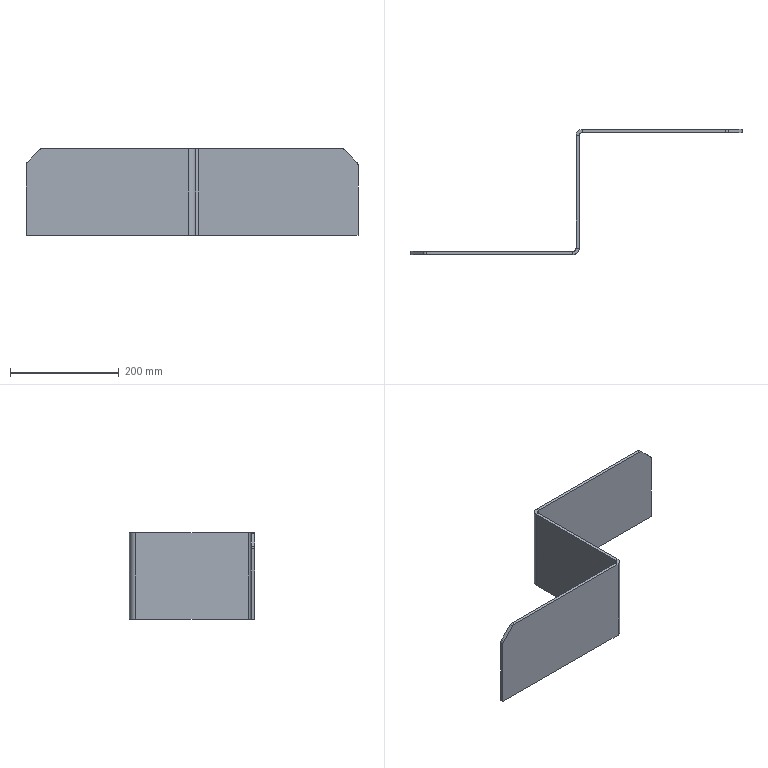Part | SolidWorks | features Chamfer 1, Fillet 1, FlatPattern 1, SMBaseFlange 1, SheetMetal 1 | 1 solid | 28 faces | box 612 x 231 x 160 mm | volume 791704 mm3 | plane 20 | cylinder 8 | commonest cylinder face diameters 14 x4 12 x2 24 x2
STEP:
#1=CARTESIAN_POINT('',(300.,0.,80.));
#2=VERTEX_POINT('',#1);
#3=CARTESIAN_POINT('',(300.,6.,80.));
#4=VERTEX_POINT('',#3);
#5=CARTESIAN_POINT('',(300.,0.,80.));
#6=DIRECTION('',(0.,1.,0.));
#7=VECTOR('',#6,1000.);
#8=LINE('',#5,#7);
#9=EDGE_CURVE('',#2,#4,#8,.T.);
#10=ORIENTED_EDGE('',*,*,#9,.F.);
#11=CARTESIAN_POINT('',(312.,12.,80.));
#12=VERTEX_POINT('',#11);
#13=CARTESIAN_POINT('',(300.,12.,80.));
#14=DIRECTION('',(0.,0.,1.));
#15=DIRECTION('',(-1.,0.,0.));
#16=AXIS2_PLACEMENT_3D('',#13,#14,#15);
#17=CIRCLE('',#16,12.);
#18=EDGE_CURVE('',#2,#12,#17,.T.);
#19=ORIENTED_EDGE('',*,*,#18,.T.);
#20=CARTESIAN_POINT('',(306.,12.,80.));
#21=VERTEX_POINT('',#20);
#22=CARTESIAN_POINT('',(306.,12.,80.));
#23=DIRECTION('',(1.,0.,0.));
#24=VECTOR('',#23,1000.);
#25=LINE('',#22,#24);
#26=EDGE_CURVE('',#21,#12,#25,.T.);
#27=ORIENTED_EDGE('',*,*,#26,.F.);
#28=CARTESIAN_POINT('',(300.,12.,80.));
#29=DIRECTION('',(0.,0.,1.));
#30=DIRECTION('',(1.,0.,0.));
#31=AXIS2_PLACEMENT_3D('',#28,#29,#30);
#32=CIRCLE('',#31,6.);
#33=EDGE_CURVE('',#4,#21,#32,.T.);
#34=ORIENTED_EDGE('',*,*,#33,.F.);
#35=EDGE_LOOP('',(#10,#19,#27,#34));
#36=FACE_OUTER_BOUND('',#35,.T.);
#37=CARTESIAN_POINT('',(300.,0.,80.));
#38=DIRECTION('',(0.,0.,1.));
#39=DIRECTION('',(1.,0.,0.));
#40=AXIS2_PLACEMENT_3D('',#37,#38,#39);
#41=PLANE('',#40);
#42=ADVANCED_FACE('',(#36),#41,.T.);
#43=CARTESIAN_POINT('',(29.899,6.,80.));
#44=VERTEX_POINT('',#43);
#45=CARTESIAN_POINT('',(0.,6.,80.));
#46=DIRECTION('',(1.,0.,0.));
#47=VECTOR('',#46,1000.);
#48=LINE('',#45,#47);
#49=EDGE_CURVE('',#44,#4,#48,.T.);
#50=ORIENTED_EDGE('',*,*,#49,.F.);
#51=CARTESIAN_POINT('',(29.899,0.,80.));
#52=VERTEX_POINT('',#51);
#53=CARTESIAN_POINT('',(29.899,12.,80.));
#54=DIRECTION('',(0.,-1.,0.));
#55=VECTOR('',#54,1000.);
#56=LINE('',#53,#55);
#57=EDGE_CURVE('',#44,#52,#56,.T.);
#58=ORIENTED_EDGE('',*,*,#57,.T.);
#59=CARTESIAN_POINT('',(0.,0.,80.));
#60=DIRECTION('',(1.,0.,0.));
#61=VECTOR('',#60,1000.);
#62=LINE('',#59,#61);
#63=EDGE_CURVE('',#52,#2,#62,.T.);
#64=ORIENTED_EDGE('',*,*,#63,.T.);
#65=ORIENTED_EDGE('',*,*,#9,.T.);
#66=EDGE_LOOP('',(#50,#58,#64,#65));
#67=FACE_OUTER_BOUND('',#66,.T.);
#68=CARTESIAN_POINT('',(306.,12.,80.));
#69=DIRECTION('',(0.,0.,1.));
#70=DIRECTION('',(1.,0.,0.));
#71=AXIS2_PLACEMENT_3D('',#68,#69,#70);
#72=PLANE('',#71);
#73=ADVANCED_FACE('',(#67),#72,.T.);
#74=CARTESIAN_POINT('',(312.,12.,-80.));
#75=VERTEX_POINT('',#74);
#76=CARTESIAN_POINT('',(306.,12.,-80.));
#77=VERTEX_POINT('',#76);
#78=CARTESIAN_POINT('',(312.,12.,-80.));
#79=DIRECTION('',(-1.,0.,0.));
#80=VECTOR('',#79,1000.);
#81=LINE('',#78,#80);
#82=EDGE_CURVE('',#75,#77,#81,.T.);
#83=ORIENTED_EDGE('',*,*,#82,.F.);
#84=CARTESIAN_POINT('',(300.,0.,-80.));
#85=VERTEX_POINT('',#84);
#86=CARTESIAN_POINT('',(300.,12.,-80.));
#87=DIRECTION('',(0.,0.,1.));
#88=DIRECTION('',(-1.,0.,0.));
#89=AXIS2_PLACEMENT_3D('',#86,#87,#88);
#90=CIRCLE('',#89,12.);
#91=EDGE_CURVE('',#85,#75,#90,.T.);
#92=ORIENTED_EDGE('',*,*,#91,.F.);
#93=CARTESIAN_POINT('',(300.,6.,-80.));
#94=VERTEX_POINT('',#93);
#95=CARTESIAN_POINT('',(300.,6.,-80.));
#96=DIRECTION('',(0.,-1.,0.));
#97=VECTOR('',#96,1000.);
#98=LINE('',#95,#97);
#99=EDGE_CURVE('',#94,#85,#98,.T.);
#100=ORIENTED_EDGE('',*,*,#99,.F.);
#101=CARTESIAN_POINT('',(300.,12.,-80.));
#102=DIRECTION('',(0.,0.,1.));
#103=DIRECTION('',(1.,0.,0.));
#104=AXIS2_PLACEMENT_3D('',#101,#102,#103);
#105=CIRCLE('',#104,6.);
#106=EDGE_CURVE('',#94,#77,#105,.T.);
#107=ORIENTED_EDGE('',*,*,#106,.T.);
#108=EDGE_LOOP('',(#83,#92,#100,#107));
#109=FACE_OUTER_BOUND('',#108,.T.);
#110=CARTESIAN_POINT('',(312.,12.,-80.));
#111=DIRECTION('',(0.,0.,-1.));
#112=DIRECTION('',(-1.,0.,0.));
#113=AXIS2_PLACEMENT_3D('',#110,#111,#112);
#114=PLANE('',#113);
#115=ADVANCED_FACE('',(#109),#114,.T.);
#116=CARTESIAN_POINT('',(312.,219.,-80.));
#117=VERTEX_POINT('',#116);
#118=CARTESIAN_POINT('',(312.,0.,-80.));
#119=DIRECTION('',(0.,1.,0.));
#120=VECTOR('',#119,1000.);
#121=LINE('',#118,#120);
#122=EDGE_CURVE('',#75,#117,#121,.T.);
#123=ORIENTED_EDGE('',*,*,#122,.F.);
#124=ORIENTED_EDGE('',*,*,#82,.T.);
#125=CARTESIAN_POINT('',(306.,219.,-80.));
#126=VERTEX_POINT('',#125);
#127=CARTESIAN_POINT('',(306.,0.,-80.));
#128=DIRECTION('',(0.,1.,0.));
#129=VECTOR('',#128,1000.);
#130=LINE('',#127,#129);
#131=EDGE_CURVE('',#77,#126,#130,.T.);
#132=ORIENTED_EDGE('',*,*,#131,.T.);
#133=CARTESIAN_POINT('',(306.,219.,-80.));
#134=DIRECTION('',(1.,0.,0.));
#135=VECTOR('',#134,1000.);
#136=LINE('',#133,#135);
#137=EDGE_CURVE('',#126,#117,#136,.T.);
#138=ORIENTED_EDGE('',*,*,#137,.T.);
#139=EDGE_LOOP('',(#123,#124,#132,#138));
#140=FACE_OUTER_BOUND('',#139,.T.);
#141=CARTESIAN_POINT('',(300.,6.,-80.));
#142=DIRECTION('',(0.,0.,-1.));
#143=DIRECTION('',(-1.,0.,0.));
#144=AXIS2_PLACEMENT_3D('',#141,#142,#143);
#145=PLANE('',#144);
#146=ADVANCED_FACE('',(#140),#145,.T.);
#147=CARTESIAN_POINT('',(312.,219.,80.));
#148=VERTEX_POINT('',#147);
#149=CARTESIAN_POINT('',(306.,219.,80.));
#150=VERTEX_POINT('',#149);
#151=CARTESIAN_POINT('',(312.,219.,80.));
#152=DIRECTION('',(-1.,0.,0.));
#153=VECTOR('',#152,1000.);
#154=LINE('',#151,#153);
#155=EDGE_CURVE('',#148,#150,#154,.T.);
#156=ORIENTED_EDGE('',*,*,#155,.F.);
#157=CARTESIAN_POINT('',(318.,225.,80.));
#158=VERTEX_POINT('',#157);
#159=CARTESIAN_POINT('',(318.,219.,80.));
#160=DIRECTION('',(0.,0.,-1.));
#161=DIRECTION('',(1.,0.,0.));
#162=AXIS2_PLACEMENT_3D('',#159,#160,#161);
#163=CIRCLE('',#162,6.);
#164=EDGE_CURVE('',#148,#158,#163,.T.);
#165=ORIENTED_EDGE('',*,*,#164,.T.);
#166=CARTESIAN_POINT('',(318.,231.,80.));
#167=VERTEX_POINT('',#166);
#168=CARTESIAN_POINT('',(318.,231.,80.));
#169=DIRECTION('',(0.,-1.,0.));
#170=VECTOR('',#169,1000.);
#171=LINE('',#168,#170);
#172=EDGE_CURVE('',#167,#158,#171,.T.);
#173=ORIENTED_EDGE('',*,*,#172,.F.);
#174=CARTESIAN_POINT('',(318.,219.,80.));
#175=DIRECTION('',(0.,0.,-1.));
#176=DIRECTION('',(1.,0.,0.));
#177=AXIS2_PLACEMENT_3D('',#174,#175,#176);
#178=CIRCLE('',#177,12.);
#179=EDGE_CURVE('',#150,#167,#178,.T.);
#180=ORIENTED_EDGE('',*,*,#179,.F.);
#181=EDGE_LOOP('',(#156,#165,#173,#180));
#182=FACE_OUTER_BOUND('',#181,.T.);
#183=CARTESIAN_POINT('',(312.,219.,80.));
#184=DIRECTION('',(0.,0.,1.));
#185=DIRECTION('',(1.,0.,0.));
#186=AXIS2_PLACEMENT_3D('',#183,#184,#185);
#187=PLANE('',#186);
#188=ADVANCED_FACE('',(#182),#187,.T.);
#189=CARTESIAN_POINT('',(312.,0.,80.));
#190=DIRECTION('',(0.,1.,0.));
#191=VECTOR('',#190,1000.);
#192=LINE('',#189,#191);
#193=EDGE_CURVE('',#12,#148,#192,.T.);
#194=ORIENTED_EDGE('',*,*,#193,.T.);
#195=ORIENTED_EDGE('',*,*,#155,.T.);
#196=CARTESIAN_POINT('',(306.,0.,80.));
#197=DIRECTION('',(0.,1.,0.));
#198=VECTOR('',#197,1000.);
#199=LINE('',#196,#198);
#200=EDGE_CURVE('',#21,#150,#199,.T.);
#201=ORIENTED_EDGE('',*,*,#200,.F.);
#202=ORIENTED_EDGE('',*,*,#26,.T.);
#203=EDGE_LOOP('',(#194,#195,#201,#202));
#204=FACE_OUTER_BOUND('',#203,.T.);
#205=CARTESIAN_POINT('',(318.,231.,80.));
#206=DIRECTION('',(0.,0.,1.));
#207=DIRECTION('',(1.,0.,0.));
#208=AXIS2_PLACEMENT_3D('',#205,#206,#207);
#209=PLANE('',#208);
#210=ADVANCED_FACE('',(#204),#209,.T.);
#211=CARTESIAN_POINT('',(318.,225.,-80.));
#212=VERTEX_POINT('',#211);
#213=CARTESIAN_POINT('',(318.,231.,-80.));
#214=VERTEX_POINT('',#213);
#215=CARTESIAN_POINT('',(318.,225.,-80.));
#216=DIRECTION('',(0.,1.,0.));
#217=VECTOR('',#216,1000.);
#218=LINE('',#215,#217);
#219=EDGE_CURVE('',#212,#214,#218,.T.);
#220=ORIENTED_EDGE('',*,*,#219,.F.);
#221=CARTESIAN_POINT('',(318.,219.,-80.));
#222=DIRECTION('',(0.,0.,-1.));
#223=DIRECTION('',(1.,0.,0.));
#224=AXIS2_PLACEMENT_3D('',#221,#222,#223);
#225=CIRCLE('',#224,6.);
#226=EDGE_CURVE('',#117,#212,#225,.T.);
#227=ORIENTED_EDGE('',*,*,#226,.F.);
#228=ORIENTED_EDGE('',*,*,#137,.F.);
#229=CARTESIAN_POINT('',(318.,219.,-80.));
#230=DIRECTION('',(0.,0.,-1.));
#231=DIRECTION('',(1.,0.,0.));
#232=AXIS2_PLACEMENT_3D('',#229,#230,#231);
#233=CIRCLE('',#232,12.);
#234=EDGE_CURVE('',#126,#214,#233,.T.);
#235=ORIENTED_EDGE('',*,*,#234,.T.);
#236=EDGE_LOOP('',(#220,#227,#228,#235));
#237=FACE_OUTER_BOUND('',#236,.T.);
#238=CARTESIAN_POINT('',(318.,225.,-80.));
#239=DIRECTION('',(0.,0.,-1.));
#240=DIRECTION('',(-1.,0.,0.));
#241=AXIS2_PLACEMENT_3D('',#238,#239,#240);
#242=PLANE('',#241);
#243=ADVANCED_FACE('',(#237),#242,.T.);
#244=CARTESIAN_POINT('',(612.,225.,-80.));
#245=VERTEX_POINT('',#244);
#246=CARTESIAN_POINT('',(312.,225.,-80.));
#247=DIRECTION('',(1.,0.,0.));
#248=VECTOR('',#247,1000.);
#249=LINE('',#246,#248);
#250=EDGE_CURVE('',#212,#245,#249,.T.);
#251=ORIENTED_EDGE('',*,*,#250,.F.);
#252=ORIENTED_EDGE('',*,*,#219,.T.);
#253=CARTESIAN_POINT('',(612.,231.,-80.));
#254=VERTEX_POINT('',#253);
#255=CARTESIAN_POINT('',(312.,231.,-80.));
#256=DIRECTION('',(1.,0.,0.));
#257=VECTOR('',#256,1000.);
#258=LINE('',#255,#257);
#259=EDGE_CURVE('',#214,#254,#258,.T.);
#260=ORIENTED_EDGE('',*,*,#259,.T.);
#261=CARTESIAN_POINT('',(612.,231.,-80.));
#262=DIRECTION('',(0.,-1.,0.));
#263=VECTOR('',#262,1000.);
#264=LINE('',#261,#263);
#265=EDGE_CURVE('',#254,#245,#264,.T.);
#266=ORIENTED_EDGE('',*,*,#265,.T.);
#267=EDGE_LOOP('',(#251,#252,#260,#266));
#268=FACE_OUTER_BOUND('',#267,.T.);
#269=CARTESIAN_POINT('',(306.,219.,-80.));
#270=DIRECTION('',(0.,0.,-1.));
#271=DIRECTION('',(-1.,0.,0.));
#272=AXIS2_PLACEMENT_3D('',#269,#270,#271);
#273=PLANE('',#272);
#274=ADVANCED_FACE('',(#268),#273,.T.);
#275=CARTESIAN_POINT('',(612.,225.,50.101));
#276=VERTEX_POINT('',#275);
#277=CARTESIAN_POINT('',(612.,225.,80.));
#278=DIRECTION('',(0.,0.,-1.));
#279=VECTOR('',#278,1000.);
#280=LINE('',#277,#279);
#281=EDGE_CURVE('',#276,#245,#280,.T.);
#282=ORIENTED_EDGE('',*,*,#281,.F.);
#283=CARTESIAN_POINT('',(609.95,225.,55.05));
#284=VERTEX_POINT('',#283);
#285=CARTESIAN_POINT('',(605.,225.,50.101));
#286=DIRECTION('',(0.,-1.,0.));
#287=DIRECTION('',(0.,0.,1.));
#288=AXIS2_PLACEMENT_3D('',#285,#286,#287);
#289=CIRCLE('',#288,7.);
#290=EDGE_CURVE('',#276,#284,#289,.T.);
#291=ORIENTED_EDGE('',*,*,#290,.T.);
#292=CARTESIAN_POINT('',(587.05,225.,77.95));
#293=VERTEX_POINT('',#292);
#294=CARTESIAN_POINT('',(612.,225.,53.));
#295=DIRECTION('',(-0.7071,0.,0.7071));
#296=VECTOR('',#295,1000.);
#297=LINE('',#294,#296);
#298=EDGE_CURVE('',#284,#293,#297,.T.);
#299=ORIENTED_EDGE('',*,*,#298,.T.);
#300=CARTESIAN_POINT('',(582.101,225.,80.));
#301=VERTEX_POINT('',#300);
#302=CARTESIAN_POINT('',(582.101,225.,73.));
#303=DIRECTION('',(0.,-1.,0.));
#304=DIRECTION('',(0.,0.,1.));
#305=AXIS2_PLACEMENT_3D('',#302,#303,#304);
#306=CIRCLE('',#305,7.);
#307=EDGE_CURVE('',#293,#301,#306,.T.);
#308=ORIENTED_EDGE('',*,*,#307,.T.);
#309=CARTESIAN_POINT('',(312.,225.,80.));
#310=DIRECTION('',(1.,0.,0.));
#311=VECTOR('',#310,1000.);
#312=LINE('',#309,#311);
#313=EDGE_CURVE('',#158,#301,#312,.T.);
#314=ORIENTED_EDGE('',*,*,#313,.F.);
#315=CARTESIAN_POINT('',(318.,225.,80.));
#316=DIRECTION('',(0.,0.,-1.));
#317=VECTOR('',#316,1000.);
#318=LINE('',#315,#317);
#319=EDGE_CURVE('',#158,#212,#318,.T.);
#320=ORIENTED_EDGE('',*,*,#319,.T.);
#321=ORIENTED_EDGE('',*,*,#250,.T.);
#322=EDGE_LOOP('',(#282,#291,#299,#308,#314,#320,#321));
#323=FACE_OUTER_BOUND('',#322,.T.);
#324=CARTESIAN_POINT('',(312.,225.,80.));
#325=DIRECTION('',(0.,1.,0.));
#326=DIRECTION('',(0.,0.,1.));
#327=AXIS2_PLACEMENT_3D('',#324,#325,#326);
#328=PLANE('',#327);
#329=ADVANCED_FACE('',(#323),#328,.F.);
#330=CARTESIAN_POINT('',(612.,231.,50.101));
#331=VERTEX_POINT('',#330);
#332=CARTESIAN_POINT('',(612.,231.,80.));
#333=DIRECTION('',(0.,0.,-1.));
#334=VECTOR('',#333,1000.);
#335=LINE('',#332,#334);
#336=EDGE_CURVE('',#331,#254,#335,.T.);
#337=ORIENTED_EDGE('',*,*,#336,.F.);
#338=CARTESIAN_POINT('',(612.,231.,50.101));
#339=DIRECTION('',(0.,-1.,0.));
#340=VECTOR('',#339,1000.);
#341=LINE('',#338,#340);
#342=EDGE_CURVE('',#331,#276,#341,.T.);
#343=ORIENTED_EDGE('',*,*,#342,.T.);
#344=ORIENTED_EDGE('',*,*,#281,.T.);
#345=ORIENTED_EDGE('',*,*,#265,.F.);
#346=EDGE_LOOP('',(#337,#343,#344,#345));
#347=FACE_OUTER_BOUND('',#346,.T.);
#348=CARTESIAN_POINT('',(612.,231.,80.));
#349=DIRECTION('',(1.,0.,0.));
#350=DIRECTION('',(0.,0.,-1.));
#351=AXIS2_PLACEMENT_3D('',#348,#349,#350);
#352=PLANE('',#351);
#353=ADVANCED_FACE('',(#347),#352,.T.);
#354=CARTESIAN_POINT('',(587.05,231.,77.95));
#355=VERTEX_POINT('',#354);
#356=CARTESIAN_POINT('',(609.95,231.,55.05));
#357=VERTEX_POINT('',#356);
#358=CARTESIAN_POINT('',(448.5,231.,216.5));
#359=DIRECTION('',(0.7071,0.,-0.7071));
#360=VECTOR('',#359,1000.);
#361=LINE('',#358,#360);
#362=EDGE_CURVE('',#355,#357,#361,.T.);
#363=ORIENTED_EDGE('',*,*,#362,.T.);
#364=CARTESIAN_POINT('',(605.,231.,50.101));
#365=DIRECTION('',(0.,1.,0.));
#366=DIRECTION('',(0.,0.,1.));
#367=AXIS2_PLACEMENT_3D('',#364,#365,#366);
#368=CIRCLE('',#367,7.);
#369=EDGE_CURVE('',#357,#331,#368,.T.);
#370=ORIENTED_EDGE('',*,*,#369,.T.);
#371=ORIENTED_EDGE('',*,*,#336,.T.);
#372=ORIENTED_EDGE('',*,*,#259,.F.);
#373=CARTESIAN_POINT('',(318.,231.,80.));
#374=DIRECTION('',(0.,0.,-1.));
#375=VECTOR('',#374,1000.);
#376=LINE('',#373,#375);
#377=EDGE_CURVE('',#167,#214,#376,.T.);
#378=ORIENTED_EDGE('',*,*,#377,.F.);
#379=CARTESIAN_POINT('',(582.101,231.,80.));
#380=VERTEX_POINT('',#379);
#381=CARTESIAN_POINT('',(312.,231.,80.));
#382=DIRECTION('',(1.,0.,0.));
#383=VECTOR('',#382,1000.);
#384=LINE('',#381,#383);
#385=EDGE_CURVE('',#167,#380,#384,.T.);
#386=ORIENTED_EDGE('',*,*,#385,.T.);
#387=CARTESIAN_POINT('',(582.101,231.,73.));
#388=DIRECTION('',(0.,1.,0.));
#389=DIRECTION('',(0.,0.,1.));
#390=AXIS2_PLACEMENT_3D('',#387,#388,#389);
#391=CIRCLE('',#390,7.);
#392=EDGE_CURVE('',#380,#355,#391,.T.);
#393=ORIENTED_EDGE('',*,*,#392,.T.);
#394=EDGE_LOOP('',(#363,#370,#371,#372,#378,#386,#393));
#395=FACE_OUTER_BOUND('',#394,.T.);
#396=CARTESIAN_POINT('',(312.,231.,80.));
#397=DIRECTION('',(0.,1.,0.));
#398=DIRECTION('',(0.,0.,1.));
#399=AXIS2_PLACEMENT_3D('',#396,#397,#398);
#400=PLANE('',#399);
#401=ADVANCED_FACE('',(#395),#400,.T.);
#402=ORIENTED_EDGE('',*,*,#234,.F.);
#403=CARTESIAN_POINT('',(306.,219.,80.));
#404=DIRECTION('',(0.,0.,-1.));
#405=VECTOR('',#404,1000.);
#406=LINE('',#403,#405);
#407=EDGE_CURVE('',#150,#126,#406,.T.);
#408=ORIENTED_EDGE('',*,*,#407,.F.);
#409=ORIENTED_EDGE('',*,*,#179,.T.);
#410=ORIENTED_EDGE('',*,*,#377,.T.);
#411=EDGE_LOOP('',(#402,#408,#409,#410));
#412=FACE_OUTER_BOUND('',#411,.T.);
#413=CARTESIAN_POINT('',(318.,219.,80.));
#414=DIRECTION('',(0.,0.,-1.));
#415=DIRECTION('',(-1.,0.,0.));
#416=AXIS2_PLACEMENT_3D('',#413,#414,#415);
#417=CYLINDRICAL_SURFACE('',#416,12.);
#418=ADVANCED_FACE('',(#412),#417,.T.);
#419=ORIENTED_EDGE('',*,*,#131,.F.);
#420=CARTESIAN_POINT('',(306.,12.,80.));
#421=DIRECTION('',(0.,0.,-1.));
#422=VECTOR('',#421,1000.);
#423=LINE('',#420,#422);
#424=EDGE_CURVE('',#21,#77,#423,.T.);
#425=ORIENTED_EDGE('',*,*,#424,.F.);
#426=ORIENTED_EDGE('',*,*,#200,.T.);
#427=ORIENTED_EDGE('',*,*,#407,.T.);
#428=EDGE_LOOP('',(#419,#425,#426,#427));
#429=FACE_OUTER_BOUND('',#428,.T.);
#430=CARTESIAN_POINT('',(306.,0.,80.));
#431=DIRECTION('',(-1.,0.,0.));
#432=DIRECTION('',(0.,0.,1.));
#433=AXIS2_PLACEMENT_3D('',#430,#431,#432);
#434=PLANE('',#433);
#435=ADVANCED_FACE('',(#429),#434,.T.);
#436=ORIENTED_EDGE('',*,*,#106,.F.);
#437=CARTESIAN_POINT('',(300.,6.,80.));
#438=DIRECTION('',(0.,0.,-1.));
#439=VECTOR('',#438,1000.);
#440=LINE('',#437,#439);
#441=EDGE_CURVE('',#4,#94,#440,.T.);
#442=ORIENTED_EDGE('',*,*,#441,.F.);
#443=ORIENTED_EDGE('',*,*,#33,.T.);
#444=ORIENTED_EDGE('',*,*,#424,.T.);
#445=EDGE_LOOP('',(#436,#442,#443,#444));
#446=FACE_OUTER_BOUND('',#445,.T.);
#447=CARTESIAN_POINT('',(300.,12.,80.));
#448=DIRECTION('',(0.,0.,-1.));
#449=DIRECTION('',(-1.,0.,0.));
#450=AXIS2_PLACEMENT_3D('',#447,#448,#449);
#451=CYLINDRICAL_SURFACE('',#450,6.);
#452=ADVANCED_FACE('',(#446),#451,.F.);
#453=CARTESIAN_POINT('',(0.,6.,50.101));
#454=VERTEX_POINT('',#453);
#455=CARTESIAN_POINT('',(0.,6.,-80.));
#456=VERTEX_POINT('',#455);
#457=CARTESIAN_POINT('',(0.,6.,80.));
#458=DIRECTION('',(0.,0.,-1.));
#459=VECTOR('',#458,1000.);
#460=LINE('',#457,#459);
#461=EDGE_CURVE('',#454,#456,#460,.T.);
#462=ORIENTED_EDGE('',*,*,#461,.F.);
#463=CARTESIAN_POINT('',(2.05,6.,55.05));
#464=VERTEX_POINT('',#463);
#465=CARTESIAN_POINT('',(7.,6.,50.101));
#466=DIRECTION('',(0.,1.,0.));
#467=DIRECTION('',(0.,0.,1.));
#468=AXIS2_PLACEMENT_3D('',#465,#466,#467);
#469=CIRCLE('',#468,7.);
#470=EDGE_CURVE('',#454,#464,#469,.T.);
#471=ORIENTED_EDGE('',*,*,#470,.T.);
#472=CARTESIAN_POINT('',(24.95,6.,77.95));
#473=VERTEX_POINT('',#472);
#474=CARTESIAN_POINT('',(13.5,6.,66.5));
#475=DIRECTION('',(0.7071,0.,0.7071));
#476=VECTOR('',#475,1000.);
#477=LINE('',#474,#476);
#478=EDGE_CURVE('',#464,#473,#477,.T.);
#479=ORIENTED_EDGE('',*,*,#478,.T.);
#480=CARTESIAN_POINT('',(29.899,6.,73.));
#481=DIRECTION('',(0.,1.,0.));
#482=DIRECTION('',(0.,0.,1.));
#483=AXIS2_PLACEMENT_3D('',#480,#481,#482);
#484=CIRCLE('',#483,7.);
#485=EDGE_CURVE('',#473,#44,#484,.T.);
#486=ORIENTED_EDGE('',*,*,#485,.T.);
#487=ORIENTED_EDGE('',*,*,#49,.T.);
#488=ORIENTED_EDGE('',*,*,#441,.T.);
#489=CARTESIAN_POINT('',(0.,6.,-80.));
#490=DIRECTION('',(1.,0.,0.));
#491=VECTOR('',#490,1000.);
#492=LINE('',#489,#491);
#493=EDGE_CURVE('',#456,#94,#492,.T.);
#494=ORIENTED_EDGE('',*,*,#493,.F.);
#495=EDGE_LOOP('',(#462,#471,#479,#486,#487,#488,#494));
#496=FACE_OUTER_BOUND('',#495,.T.);
#497=CARTESIAN_POINT('',(0.,6.,80.));
#498=DIRECTION('',(0.,1.,0.));
#499=DIRECTION('',(0.,0.,1.));
#500=AXIS2_PLACEMENT_3D('',#497,#498,#499);
#501=PLANE('',#500);
#502=ADVANCED_FACE('',(#496),#501,.T.);
#503=CARTESIAN_POINT('',(0.,0.,50.101));
#504=VERTEX_POINT('',#503);
#505=CARTESIAN_POINT('',(0.,0.,-80.));
#506=VERTEX_POINT('',#505);
#507=CARTESIAN_POINT('',(0.,0.,80.));
#508=DIRECTION('',(0.,0.,-1.));
#509=VECTOR('',#508,1000.);
#510=LINE('',#507,#509);
#511=EDGE_CURVE('',#504,#506,#510,.T.);
#512=ORIENTED_EDGE('',*,*,#511,.F.);
#513=CARTESIAN_POINT('',(0.,0.,50.101));
#514=DIRECTION('',(0.,1.,0.));
#515=VECTOR('',#514,1000.);
#516=LINE('',#513,#515);
#517=EDGE_CURVE('',#504,#454,#516,.T.);
#518=ORIENTED_EDGE('',*,*,#517,.T.);
#519=ORIENTED_EDGE('',*,*,#461,.T.);
#520=CARTESIAN_POINT('',(0.,0.,-80.));
#521=DIRECTION('',(0.,1.,0.));
#522=VECTOR('',#521,1000.);
#523=LINE('',#520,#522);
#524=EDGE_CURVE('',#506,#456,#523,.T.);
#525=ORIENTED_EDGE('',*,*,#524,.F.);
#526=EDGE_LOOP('',(#512,#518,#519,#525));
#527=FACE_OUTER_BOUND('',#526,.T.);
#528=CARTESIAN_POINT('',(0.,0.,80.));
#529=DIRECTION('',(-1.,0.,0.));
#530=DIRECTION('',(0.,0.,1.));
#531=AXIS2_PLACEMENT_3D('',#528,#529,#530);
#532=PLANE('',#531);
#533=ADVANCED_FACE('',(#527),#532,.T.);
#534=CARTESIAN_POINT('',(24.95,0.,77.95));
#535=VERTEX_POINT('',#534);
#536=CARTESIAN_POINT('',(2.05,0.,55.05));
#537=VERTEX_POINT('',#536);
#538=CARTESIAN_POINT('',(0.,0.,53.));
#539=DIRECTION('',(-0.7071,0.,-0.7071));
#540=VECTOR('',#539,1000.);
#541=LINE('',#538,#540);
#542=EDGE_CURVE('',#535,#537,#541,.T.);
#543=ORIENTED_EDGE('',*,*,#542,.T.);
#544=CARTESIAN_POINT('',(7.,0.,50.101));
#545=DIRECTION('',(0.,-1.,0.));
#546=DIRECTION('',(0.,0.,1.));
#547=AXIS2_PLACEMENT_3D('',#544,#545,#546);
#548=CIRCLE('',#547,7.);
#549=EDGE_CURVE('',#537,#504,#548,.T.);
#550=ORIENTED_EDGE('',*,*,#549,.T.);
#551=ORIENTED_EDGE('',*,*,#511,.T.);
#552=CARTESIAN_POINT('',(0.,0.,-80.));
#553=DIRECTION('',(1.,0.,0.));
#554=VECTOR('',#553,1000.);
#555=LINE('',#552,#554);
#556=EDGE_CURVE('',#506,#85,#555,.T.);
#557=ORIENTED_EDGE('',*,*,#556,.T.);
#558=CARTESIAN_POINT('',(300.,0.,80.));
#559=DIRECTION('',(0.,0.,-1.));
#560=VECTOR('',#559,1000.);
#561=LINE('',#558,#560);
#562=EDGE_CURVE('',#2,#85,#561,.T.);
#563=ORIENTED_EDGE('',*,*,#562,.F.);
#564=ORIENTED_EDGE('',*,*,#63,.F.);
#565=CARTESIAN_POINT('',(29.899,0.,73.));
#566=DIRECTION('',(0.,-1.,0.));
#567=DIRECTION('',(0.,0.,1.));
#568=AXIS2_PLACEMENT_3D('',#565,#566,#567);
#569=CIRCLE('',#568,7.);
#570=EDGE_CURVE('',#52,#535,#569,.T.);
#571=ORIENTED_EDGE('',*,*,#570,.T.);
#572=EDGE_LOOP('',(#543,#550,#551,#557,#563,#564,#571));
#573=FACE_OUTER_BOUND('',#572,.T.);
#574=CARTESIAN_POINT('',(0.,0.,80.));
#575=DIRECTION('',(0.,1.,0.));
#576=DIRECTION('',(0.,0.,1.));
#577=AXIS2_PLACEMENT_3D('',#574,#575,#576);
#578=PLANE('',#577);
#579=ADVANCED_FACE('',(#573),#578,.F.);
#580=ORIENTED_EDGE('',*,*,#91,.T.);
#581=CARTESIAN_POINT('',(312.,12.,80.));
#582=DIRECTION('',(0.,0.,-1.));
#583=VECTOR('',#582,1000.);
#584=LINE('',#581,#583);
#585=EDGE_CURVE('',#12,#75,#584,.T.);
#586=ORIENTED_EDGE('',*,*,#585,.F.);
#587=ORIENTED_EDGE('',*,*,#18,.F.);
#588=ORIENTED_EDGE('',*,*,#562,.T.);
#589=EDGE_LOOP('',(#580,#586,#587,#588));
#590=FACE_OUTER_BOUND('',#589,.T.);
#591=CARTESIAN_POINT('',(300.,12.,80.));
#592=DIRECTION('',(0.,0.,-1.));
#593=DIRECTION('',(-1.,0.,0.));
#594=AXIS2_PLACEMENT_3D('',#591,#592,#593);
#595=CYLINDRICAL_SURFACE('',#594,12.);
#596=ADVANCED_FACE('',(#590),#595,.T.);
#597=ORIENTED_EDGE('',*,*,#122,.T.);
#598=CARTESIAN_POINT('',(312.,219.,80.));
#599=DIRECTION('',(0.,0.,-1.));
#600=VECTOR('',#599,1000.);
#601=LINE('',#598,#600);
#602=EDGE_CURVE('',#148,#117,#601,.T.);
#603=ORIENTED_EDGE('',*,*,#602,.F.);
#604=ORIENTED_EDGE('',*,*,#193,.F.);
#605=ORIENTED_EDGE('',*,*,#585,.T.);
#606=EDGE_LOOP('',(#597,#603,#604,#605));
#607=FACE_OUTER_BOUND('',#606,.T.);
#608=CARTESIAN_POINT('',(312.,0.,80.));
#609=DIRECTION('',(-1.,0.,0.));
#610=DIRECTION('',(0.,0.,1.));
#611=AXIS2_PLACEMENT_3D('',#608,#609,#610);
#612=PLANE('',#611);
#613=ADVANCED_FACE('',(#607),#612,.F.);
#614=ORIENTED_EDGE('',*,*,#226,.T.);
#615=ORIENTED_EDGE('',*,*,#319,.F.);
#616=ORIENTED_EDGE('',*,*,#164,.F.);
#617=ORIENTED_EDGE('',*,*,#602,.T.);
#618=EDGE_LOOP('',(#614,#615,#616,#617));
#619=FACE_OUTER_BOUND('',#618,.T.);
#620=CARTESIAN_POINT('',(318.,219.,80.));
#621=DIRECTION('',(0.,0.,-1.));
#622=DIRECTION('',(-1.,0.,0.));
#623=AXIS2_PLACEMENT_3D('',#620,#621,#622);
#624=CYLINDRICAL_SURFACE('',#623,6.);
#625=ADVANCED_FACE('',(#619),#624,.F.);
#626=ORIENTED_EDGE('',*,*,#313,.T.);
#627=CARTESIAN_POINT('',(582.101,219.,80.));
#628=DIRECTION('',(0.,1.,0.));
#629=VECTOR('',#628,1000.);
#630=LINE('',#627,#629);
#631=EDGE_CURVE('',#301,#380,#630,.T.);
#632=ORIENTED_EDGE('',*,*,#631,.T.);
#633=ORIENTED_EDGE('',*,*,#385,.F.);
#634=ORIENTED_EDGE('',*,*,#172,.T.);
#635=EDGE_LOOP('',(#626,#632,#633,#634));
#636=FACE_OUTER_BOUND('',#635,.T.);
#637=CARTESIAN_POINT('',(318.,219.,80.));
#638=DIRECTION('',(0.,0.,1.));
#639=DIRECTION('',(1.,0.,0.));
#640=AXIS2_PLACEMENT_3D('',#637,#638,#639);
#641=PLANE('',#640);
#642=ADVANCED_FACE('',(#636),#641,.T.);
#643=ORIENTED_EDGE('',*,*,#493,.T.);
#644=ORIENTED_EDGE('',*,*,#99,.T.);
#645=ORIENTED_EDGE('',*,*,#556,.F.);
#646=ORIENTED_EDGE('',*,*,#524,.T.);
#647=EDGE_LOOP('',(#643,#644,#645,#646));
#648=FACE_OUTER_BOUND('',#647,.T.);
#649=CARTESIAN_POINT('',(318.,219.,-80.));
#650=DIRECTION('',(0.,0.,1.));
#651=DIRECTION('',(1.,0.,0.));
#652=AXIS2_PLACEMENT_3D('',#649,#650,#651);
#653=PLANE('',#652);
#654=ADVANCED_FACE('',(#648),#653,.F.);
#655=ORIENTED_EDGE('',*,*,#298,.F.);
#656=CARTESIAN_POINT('',(609.95,231.,55.05));
#657=DIRECTION('',(0.,1.,0.));
#658=VECTOR('',#657,1000.);
#659=LINE('',#656,#658);
#660=EDGE_CURVE('',#284,#357,#659,.T.);
#661=ORIENTED_EDGE('',*,*,#660,.T.);
#662=ORIENTED_EDGE('',*,*,#362,.F.);
#663=CARTESIAN_POINT('',(587.05,231.,77.95));
#664=DIRECTION('',(0.,-1.,0.));
#665=VECTOR('',#664,1000.);
#666=LINE('',#663,#665);
#667=EDGE_CURVE('',#355,#293,#666,.T.);
#668=ORIENTED_EDGE('',*,*,#667,.T.);
#669=EDGE_LOOP('',(#655,#661,#662,#668));
#670=FACE_OUTER_BOUND('',#669,.T.);
#671=CARTESIAN_POINT('',(612.,231.,53.));
#672=DIRECTION('',(-0.7071,0.,-0.7071));
#673=DIRECTION('',(0.,-1.,0.));
#674=AXIS2_PLACEMENT_3D('',#671,#672,#673);
#675=PLANE('',#674);
#676=ADVANCED_FACE('',(#670),#675,.F.);
#677=ORIENTED_EDGE('',*,*,#478,.F.);
#678=CARTESIAN_POINT('',(2.05,0.,55.05));
#679=DIRECTION('',(0.,-1.,0.));
#680=VECTOR('',#679,1000.);
#681=LINE('',#678,#680);
#682=EDGE_CURVE('',#464,#537,#681,.T.);
#683=ORIENTED_EDGE('',*,*,#682,.T.);
#684=ORIENTED_EDGE('',*,*,#542,.F.);
#685=CARTESIAN_POINT('',(24.95,0.,77.95));
#686=DIRECTION('',(0.,1.,0.));
#687=VECTOR('',#686,1000.);
#688=LINE('',#685,#687);
#689=EDGE_CURVE('',#535,#473,#688,.T.);
#690=ORIENTED_EDGE('',*,*,#689,.T.);
#691=EDGE_LOOP('',(#677,#683,#684,#690));
#692=FACE_OUTER_BOUND('',#691,.T.);
#693=CARTESIAN_POINT('',(0.,0.,53.));
#694=DIRECTION('',(0.7071,0.,-0.7071));
#695=DIRECTION('',(0.,1.,0.));
#696=AXIS2_PLACEMENT_3D('',#693,#694,#695);
#697=PLANE('',#696);
#698=ADVANCED_FACE('',(#692),#697,.F.);
#699=ORIENTED_EDGE('',*,*,#369,.F.);
#700=ORIENTED_EDGE('',*,*,#660,.F.);
#701=ORIENTED_EDGE('',*,*,#290,.F.);
#702=ORIENTED_EDGE('',*,*,#342,.F.);
#703=EDGE_LOOP('',(#699,#700,#701,#702));
#704=FACE_OUTER_BOUND('',#703,.T.);
#705=CARTESIAN_POINT('',(605.,231.,50.101));
#706=DIRECTION('',(0.,1.,0.));
#707=DIRECTION('',(0.,0.,1.));
#708=AXIS2_PLACEMENT_3D('',#705,#706,#707);
#709=CYLINDRICAL_SURFACE('',#708,7.);
#710=ADVANCED_FACE('',(#704),#709,.T.);
#711=ORIENTED_EDGE('',*,*,#307,.F.);
#712=ORIENTED_EDGE('',*,*,#667,.F.);
#713=ORIENTED_EDGE('',*,*,#392,.F.);
#714=ORIENTED_EDGE('',*,*,#631,.F.);
#715=EDGE_LOOP('',(#711,#712,#713,#714));
#716=FACE_OUTER_BOUND('',#715,.T.);
#717=CARTESIAN_POINT('',(582.101,219.,73.));
#718=DIRECTION('',(0.,-1.,0.));
#719=DIRECTION('',(0.,0.,-1.));
#720=AXIS2_PLACEMENT_3D('',#717,#718,#719);
#721=CYLINDRICAL_SURFACE('',#720,7.);
#722=ADVANCED_FACE('',(#716),#721,.T.);
#723=ORIENTED_EDGE('',*,*,#549,.F.);
#724=ORIENTED_EDGE('',*,*,#682,.F.);
#725=ORIENTED_EDGE('',*,*,#470,.F.);
#726=ORIENTED_EDGE('',*,*,#517,.F.);
#727=EDGE_LOOP('',(#723,#724,#725,#726));
#728=FACE_OUTER_BOUND('',#727,.T.);
#729=CARTESIAN_POINT('',(7.,0.,50.101));
#730=DIRECTION('',(0.,-1.,0.));
#731=DIRECTION('',(0.,0.,-1.));
#732=AXIS2_PLACEMENT_3D('',#729,#730,#731);
#733=CYLINDRICAL_SURFACE('',#732,7.);
#734=ADVANCED_FACE('',(#728),#733,.T.);
#735=ORIENTED_EDGE('',*,*,#485,.F.);
#736=ORIENTED_EDGE('',*,*,#689,.F.);
#737=ORIENTED_EDGE('',*,*,#570,.F.);
#738=ORIENTED_EDGE('',*,*,#57,.F.);
#739=EDGE_LOOP('',(#735,#736,#737,#738));
#740=FACE_OUTER_BOUND('',#739,.T.);
#741=CARTESIAN_POINT('',(29.899,12.,73.));
#742=DIRECTION('',(0.,1.,0.));
#743=DIRECTION('',(0.,0.,1.));
#744=AXIS2_PLACEMENT_3D('',#741,#742,#743);
#745=CYLINDRICAL_SURFACE('',#744,7.);
#746=ADVANCED_FACE('',(#740),#745,.T.);
#747=CLOSED_SHELL('',(#42,#73,#115,#146,#188,#210,#243,#274,#329,#353,#401,#418,#435,#452,#502,#533,#579,#596,#613,#625,#642,#654,#676,#698,#710,#722,#734,#746));
#748=MANIFOLD_SOLID_BREP('',#747);
#749=CARTESIAN_POINT('',(0.,0.,0.));
#750=DIRECTION('',(0.,0.,1.));
#751=DIRECTION('',(1.,0.,0.));
#752=AXIS2_PLACEMENT_3D('',#749,#750,#751);
#753=(LENGTH_UNIT()NAMED_UNIT(*)SI_UNIT(.MILLI.,.METRE.));
#754=UNCERTAINTY_MEASURE_WITH_UNIT(LENGTH_MEASURE(0.00001),#753,'','');
#755=(NAMED_UNIT(*)PLANE_ANGLE_UNIT()SI_UNIT($,.RADIAN.));
#756=(NAMED_UNIT(*)SI_UNIT($,.STERADIAN.)SOLID_ANGLE_UNIT());
#757=(GEOMETRIC_REPRESENTATION_CONTEXT(3)GLOBAL_UNCERTAINTY_ASSIGNED_CONTEXT((#754))GLOBAL_UNIT_ASSIGNED_CONTEXT((#753,#755,#756))REPRESENTATION_CONTEXT('',''));
#758=ADVANCED_BREP_SHAPE_REPRESENTATION('',(#748,#752),#757);